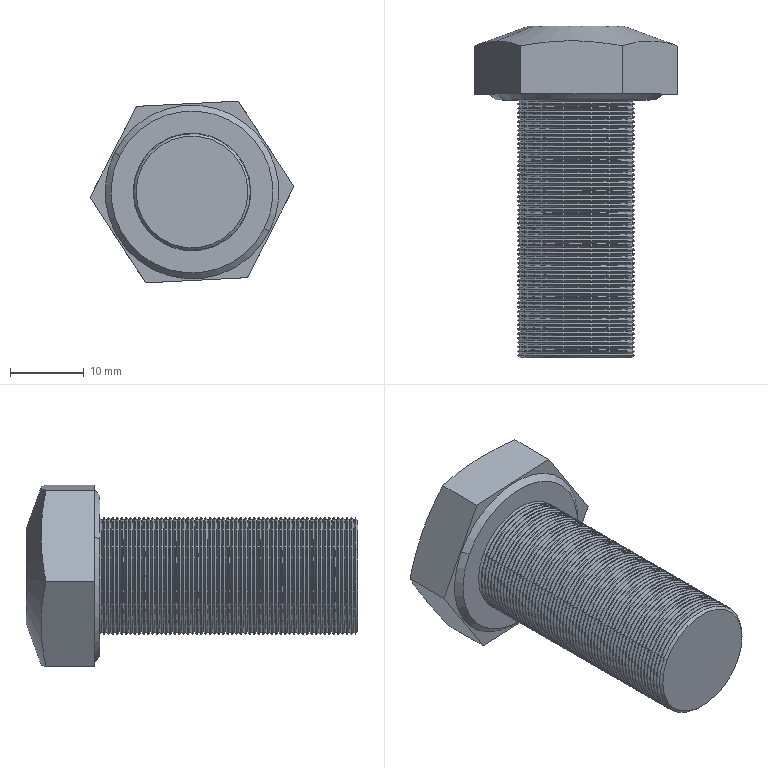Part | STEP file | 2026.6.15-Main Assembly图.sldasm-Part-79 | 1 solid | 362 faces | box 27.676 x 45 x 24.678 mm | volume 11185 mm3 | cone 238 | cylinder 114 | plane 10 | commonest cylinder face diameters 16 x114